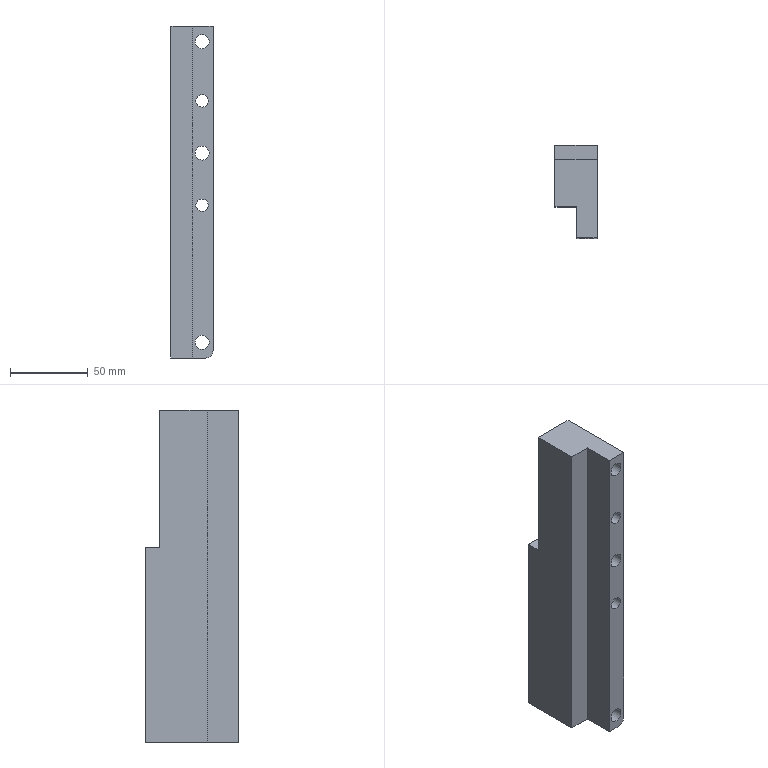Part | STEP file | SLIDE2-PLATE_id562_x_t | 1 solid | 27 faces | box 27 x 59.5 x 213.003 mm | volume 241757 mm3 | plane 18 | cylinder 9 | commonest cylinder face diameters 9 x3 14 x3 8 x2 10 x1
STEP:
#1=CARTESIAN_POINT('',(64.,-40.,62.));
#2=VERTEX_POINT('',#1);
#3=CARTESIAN_POINT('',(64.,-40.,275.003));
#4=VERTEX_POINT('',#3);
#5=CARTESIAN_POINT('',(64.,-40.,275.003));
#6=DIRECTION('',(0.,0.,1.));
#7=VECTOR('',#6,1.);
#8=LINE('',#5,#7);
#9=EDGE_CURVE('',#2,#4,#8,.T.);
#10=ORIENTED_EDGE('',*,*,#9,.T.);
#11=CARTESIAN_POINT('',(50.,-40.,275.003));
#12=VERTEX_POINT('',#11);
#13=CARTESIAN_POINT('',(-89.,-40.,275.003));
#14=DIRECTION('',(1.,0.,0.));
#15=VECTOR('',#14,1.);
#16=LINE('',#13,#15);
#17=EDGE_CURVE('',#12,#4,#16,.T.);
#18=ORIENTED_EDGE('',*,*,#17,.F.);
#19=CARTESIAN_POINT('',(50.,-40.,62.));
#20=VERTEX_POINT('',#19);
#21=CARTESIAN_POINT('',(50.,-40.,47.));
#22=DIRECTION('',(0.,0.,1.));
#23=VECTOR('',#22,1.);
#24=LINE('',#21,#23);
#25=EDGE_CURVE('',#20,#12,#24,.T.);
#26=ORIENTED_EDGE('',*,*,#25,.F.);
#27=CARTESIAN_POINT('',(50.,-40.,62.));
#28=DIRECTION('',(1.,0.,0.));
#29=VECTOR('',#28,1.);
#30=LINE('',#27,#29);
#31=EDGE_CURVE('',#20,#2,#30,.T.);
#32=ORIENTED_EDGE('',*,*,#31,.T.);
#33=EDGE_LOOP('',(#10,#18,#26,#32));
#34=FACE_OUTER_BOUND('',#33,.T.);
#35=CARTESIAN_POINT('',(64.,-40.,275.003));
#36=DIRECTION('',(0.,1.,0.));
#37=DIRECTION('',(0.,0.,1.));
#38=AXIS2_PLACEMENT_3D('',#35,#36,#37);
#39=PLANE('',#38);
#40=ADVANCED_FACE('',(#34),#39,.F.);
#41=ORIENTED_EDGE('',*,*,#9,.F.);
#42=CARTESIAN_POINT('',(64.,-60.,62.));
#43=VERTEX_POINT('',#42);
#44=CARTESIAN_POINT('',(64.,-50.,62.));
#45=DIRECTION('',(0.,-1.,0.));
#46=VECTOR('',#45,1.);
#47=LINE('',#44,#46);
#48=EDGE_CURVE('',#2,#43,#47,.T.);
#49=ORIENTED_EDGE('',*,*,#48,.T.);
#50=CARTESIAN_POINT('',(64.,-60.,275.003));
#51=VERTEX_POINT('',#50);
#52=CARTESIAN_POINT('',(64.,-60.,47.));
#53=DIRECTION('',(0.,0.,-1.));
#54=VECTOR('',#53,1.);
#55=LINE('',#52,#54);
#56=EDGE_CURVE('',#51,#43,#55,.T.);
#57=ORIENTED_EDGE('',*,*,#56,.F.);
#58=CARTESIAN_POINT('',(64.,0.5,275.003));
#59=DIRECTION('',(0.,-1.,0.));
#60=VECTOR('',#59,1.);
#61=LINE('',#58,#60);
#62=EDGE_CURVE('',#4,#51,#61,.T.);
#63=ORIENTED_EDGE('',*,*,#62,.F.);
#64=EDGE_LOOP('',(#41,#49,#57,#63));
#65=FACE_OUTER_BOUND('',#64,.T.);
#66=CARTESIAN_POINT('',(64.,-60.,275.003));
#67=DIRECTION('',(1.,0.,0.));
#68=DIRECTION('',(0.,0.,-1.));
#69=AXIS2_PLACEMENT_3D('',#66,#67,#68);
#70=PLANE('',#69);
#71=ADVANCED_FACE('',(#65),#70,.F.);
#72=CARTESIAN_POINT('',(70.,-60.,76.5));
#73=VERTEX_POINT('',#72);
#74=CARTESIAN_POINT('',(70.,-60.,72.));
#75=DIRECTION('',(0.,1.,0.));
#76=DIRECTION('',(0.,0.,1.));
#77=AXIS2_PLACEMENT_3D('',#74,#75,#76);
#78=CIRCLE('',#77,4.5);
#79=EDGE_CURVE('',#73,#73,#78,.T.);
#80=ORIENTED_EDGE('',*,*,#79,.F.);
#81=EDGE_LOOP('',(#80));
#82=FACE_BOUND('',#81,.T.);
#83=CARTESIAN_POINT('',(70.,-9.5,76.5));
#84=VERTEX_POINT('',#83);
#85=CARTESIAN_POINT('',(70.,-9.5,72.));
#86=DIRECTION('',(0.,-1.,0.));
#87=DIRECTION('',(0.,0.,1.));
#88=AXIS2_PLACEMENT_3D('',#85,#86,#87);
#89=CIRCLE('',#88,4.5);
#90=EDGE_CURVE('',#84,#84,#89,.T.);
#91=ORIENTED_EDGE('',*,*,#90,.F.);
#92=EDGE_LOOP('',(#91));
#93=FACE_BOUND('',#92,.T.);
#94=CARTESIAN_POINT('',(70.,-0.5,72.));
#95=DIRECTION('',(0.,1.,0.));
#96=DIRECTION('',(0.,0.,1.));
#97=AXIS2_PLACEMENT_3D('',#94,#95,#96);
#98=CYLINDRICAL_SURFACE('',#97,4.5);
#99=ADVANCED_FACE('',(#82,#93),#98,.F.);
#100=CARTESIAN_POINT('',(70.,-9.5,65.));
#101=VERTEX_POINT('',#100);
#102=CARTESIAN_POINT('',(70.,-9.5,79.));
#103=VERTEX_POINT('',#102);
#104=CARTESIAN_POINT('',(70.,-9.5,72.));
#105=DIRECTION('',(0.,1.,0.));
#106=DIRECTION('',(0.,0.,1.));
#107=AXIS2_PLACEMENT_3D('',#104,#105,#106);
#108=CIRCLE('',#107,7.);
#109=EDGE_CURVE('',#101,#103,#108,.T.);
#110=ORIENTED_EDGE('',*,*,#109,.F.);
#111=CARTESIAN_POINT('',(70.,-0.5,65.));
#112=VERTEX_POINT('',#111);
#113=CARTESIAN_POINT('',(70.,-0.5,65.));
#114=DIRECTION('',(0.,1.,0.));
#115=VECTOR('',#114,1.);
#116=LINE('',#113,#115);
#117=EDGE_CURVE('',#101,#112,#116,.T.);
#118=ORIENTED_EDGE('',*,*,#117,.T.);
#119=CARTESIAN_POINT('',(70.,-0.5,79.));
#120=VERTEX_POINT('',#119);
#121=CARTESIAN_POINT('',(70.,-0.5,72.));
#122=DIRECTION('',(0.,-1.,0.));
#123=DIRECTION('',(0.,0.,1.));
#124=AXIS2_PLACEMENT_3D('',#121,#122,#123);
#125=CIRCLE('',#124,7.);
#126=EDGE_CURVE('',#120,#112,#125,.T.);
#127=ORIENTED_EDGE('',*,*,#126,.F.);
#128=CARTESIAN_POINT('',(70.,-0.5,79.));
#129=DIRECTION('',(0.,-1.,0.));
#130=VECTOR('',#129,1.);
#131=LINE('',#128,#130);
#132=EDGE_CURVE('',#120,#103,#131,.T.);
#133=ORIENTED_EDGE('',*,*,#132,.T.);
#134=EDGE_LOOP('',(#110,#118,#127,#133));
#135=FACE_OUTER_BOUND('',#134,.T.);
#136=CARTESIAN_POINT('',(70.,-0.5,72.));
#137=DIRECTION('',(0.,1.,0.));
#138=DIRECTION('',(0.,0.,1.));
#139=AXIS2_PLACEMENT_3D('',#136,#137,#138);
#140=CYLINDRICAL_SURFACE('',#139,7.);
#141=ADVANCED_FACE('',(#135),#140,.F.);
#142=CARTESIAN_POINT('',(76.583,-9.5,65.));
#143=VERTEX_POINT('',#142);
#144=CARTESIAN_POINT('',(50.,-9.5,65.));
#145=DIRECTION('',(-1.,0.,0.));
#146=VECTOR('',#145,1.);
#147=LINE('',#144,#146);
#148=EDGE_CURVE('',#143,#101,#147,.T.);
#149=ORIENTED_EDGE('',*,*,#148,.F.);
#150=CARTESIAN_POINT('',(76.583,-0.5,65.));
#151=VERTEX_POINT('',#150);
#152=CARTESIAN_POINT('',(76.583,-0.5,65.));
#153=DIRECTION('',(0.,-1.,0.));
#154=VECTOR('',#153,1.);
#155=LINE('',#152,#154);
#156=EDGE_CURVE('',#151,#143,#155,.T.);
#157=ORIENTED_EDGE('',*,*,#156,.F.);
#158=CARTESIAN_POINT('',(73.,-0.5,65.));
#159=DIRECTION('',(1.,0.,0.));
#160=VECTOR('',#159,1.);
#161=LINE('',#158,#160);
#162=EDGE_CURVE('',#112,#151,#161,.T.);
#163=ORIENTED_EDGE('',*,*,#162,.F.);
#164=ORIENTED_EDGE('',*,*,#117,.F.);
#165=EDGE_LOOP('',(#149,#157,#163,#164));
#166=FACE_OUTER_BOUND('',#165,.T.);
#167=CARTESIAN_POINT('',(77.,-0.5,65.));
#168=DIRECTION('',(0.,0.,-1.));
#169=DIRECTION('',(-1.,0.,0.));
#170=AXIS2_PLACEMENT_3D('',#167,#168,#169);
#171=PLANE('',#170);
#172=ADVANCED_FACE('',(#166),#171,.F.);
#173=CARTESIAN_POINT('',(50.,-0.5,62.));
#174=VERTEX_POINT('',#173);
#175=CARTESIAN_POINT('',(50.,-0.5,62.));
#176=DIRECTION('',(0.,-1.,0.));
#177=VECTOR('',#176,1.);
#178=LINE('',#175,#177);
#179=EDGE_CURVE('',#174,#20,#178,.T.);
#180=ORIENTED_EDGE('',*,*,#179,.F.);
#181=CARTESIAN_POINT('',(72.,-0.5,62.));
#182=VERTEX_POINT('',#181);
#183=CARTESIAN_POINT('',(73.,-0.5,62.));
#184=DIRECTION('',(-1.,0.,0.));
#185=VECTOR('',#184,1.);
#186=LINE('',#183,#185);
#187=EDGE_CURVE('',#182,#174,#186,.T.);
#188=ORIENTED_EDGE('',*,*,#187,.F.);
#189=CARTESIAN_POINT('',(72.,-60.,62.));
#190=VERTEX_POINT('',#189);
#191=CARTESIAN_POINT('',(72.,-0.5,62.));
#192=DIRECTION('',(0.,1.,0.));
#193=VECTOR('',#192,1.);
#194=LINE('',#191,#193);
#195=EDGE_CURVE('',#190,#182,#194,.T.);
#196=ORIENTED_EDGE('',*,*,#195,.F.);
#197=CARTESIAN_POINT('',(58.,-60.,62.));
#198=DIRECTION('',(1.,0.,0.));
#199=VECTOR('',#198,1.);
#200=LINE('',#197,#199);
#201=EDGE_CURVE('',#43,#190,#200,.T.);
#202=ORIENTED_EDGE('',*,*,#201,.F.);
#203=ORIENTED_EDGE('',*,*,#48,.F.);
#204=ORIENTED_EDGE('',*,*,#31,.F.);
#205=EDGE_LOOP('',(#180,#188,#196,#202,#203,#204));
#206=FACE_OUTER_BOUND('',#205,.T.);
#207=CARTESIAN_POINT('',(50.,-50.,62.));
#208=DIRECTION('',(0.,0.,1.));
#209=DIRECTION('',(1.,0.,0.));
#210=AXIS2_PLACEMENT_3D('',#207,#208,#209);
#211=PLANE('',#210);
#212=ADVANCED_FACE('',(#206),#211,.F.);
#213=CARTESIAN_POINT('',(70.,-0.5,164.));
#214=VERTEX_POINT('',#213);
#215=CARTESIAN_POINT('',(70.,-0.5,160.));
#216=DIRECTION('',(0.,-1.,0.));
#217=DIRECTION('',(0.,0.,1.));
#218=AXIS2_PLACEMENT_3D('',#215,#216,#217);
#219=CIRCLE('',#218,4.);
#220=EDGE_CURVE('',#214,#214,#219,.T.);
#221=ORIENTED_EDGE('',*,*,#220,.F.);
#222=EDGE_LOOP('',(#221));
#223=FACE_BOUND('',#222,.T.);
#224=CARTESIAN_POINT('',(70.,-60.,164.));
#225=VERTEX_POINT('',#224);
#226=CARTESIAN_POINT('',(70.,-60.,160.));
#227=DIRECTION('',(0.,1.,0.));
#228=DIRECTION('',(0.,0.,1.));
#229=AXIS2_PLACEMENT_3D('',#226,#227,#228);
#230=CIRCLE('',#229,4.);
#231=EDGE_CURVE('',#225,#225,#230,.T.);
#232=ORIENTED_EDGE('',*,*,#231,.F.);
#233=EDGE_LOOP('',(#232));
#234=FACE_BOUND('',#233,.T.);
#235=CARTESIAN_POINT('',(70.,-0.5,160.));
#236=DIRECTION('',(0.,1.,0.));
#237=DIRECTION('',(0.,0.,1.));
#238=AXIS2_PLACEMENT_3D('',#235,#236,#237);
#239=CYLINDRICAL_SURFACE('',#238,4.);
#240=ADVANCED_FACE('',(#223,#234),#239,.F.);
#241=CARTESIAN_POINT('',(70.,-60.,198.003));
#242=VERTEX_POINT('',#241);
#243=CARTESIAN_POINT('',(70.,-60.,193.503));
#244=DIRECTION('',(0.,1.,0.));
#245=DIRECTION('',(0.,0.,1.));
#246=AXIS2_PLACEMENT_3D('',#243,#244,#245);
#247=CIRCLE('',#246,4.5);
#248=EDGE_CURVE('',#242,#242,#247,.T.);
#249=ORIENTED_EDGE('',*,*,#248,.F.);
#250=EDGE_LOOP('',(#249));
#251=FACE_BOUND('',#250,.T.);
#252=CARTESIAN_POINT('',(70.,-19.5,198.003));
#253=VERTEX_POINT('',#252);
#254=CARTESIAN_POINT('',(70.,-19.5,193.503));
#255=DIRECTION('',(0.,-1.,0.));
#256=DIRECTION('',(0.,0.,1.));
#257=AXIS2_PLACEMENT_3D('',#254,#255,#256);
#258=CIRCLE('',#257,4.5);
#259=EDGE_CURVE('',#253,#253,#258,.T.);
#260=ORIENTED_EDGE('',*,*,#259,.F.);
#261=EDGE_LOOP('',(#260));
#262=FACE_BOUND('',#261,.T.);
#263=CARTESIAN_POINT('',(70.,-0.5,193.503));
#264=DIRECTION('',(0.,1.,0.));
#265=DIRECTION('',(0.,0.,1.));
#266=AXIS2_PLACEMENT_3D('',#263,#264,#265);
#267=CYLINDRICAL_SURFACE('',#266,4.5);
#268=ADVANCED_FACE('',(#251,#262),#267,.F.);
#269=CARTESIAN_POINT('',(70.,-60.,269.503));
#270=VERTEX_POINT('',#269);
#271=CARTESIAN_POINT('',(70.,-60.,265.003));
#272=DIRECTION('',(0.,1.,0.));
#273=DIRECTION('',(0.,0.,1.));
#274=AXIS2_PLACEMENT_3D('',#271,#272,#273);
#275=CIRCLE('',#274,4.5);
#276=EDGE_CURVE('',#270,#270,#275,.T.);
#277=ORIENTED_EDGE('',*,*,#276,.F.);
#278=EDGE_LOOP('',(#277));
#279=FACE_BOUND('',#278,.T.);
#280=CARTESIAN_POINT('',(70.,-19.5,269.503));
#281=VERTEX_POINT('',#280);
#282=CARTESIAN_POINT('',(70.,-19.5,265.003));
#283=DIRECTION('',(0.,-1.,0.));
#284=DIRECTION('',(0.,0.,1.));
#285=AXIS2_PLACEMENT_3D('',#282,#283,#284);
#286=CIRCLE('',#285,4.5);
#287=EDGE_CURVE('',#281,#281,#286,.T.);
#288=ORIENTED_EDGE('',*,*,#287,.F.);
#289=EDGE_LOOP('',(#288));
#290=FACE_BOUND('',#289,.T.);
#291=CARTESIAN_POINT('',(70.,-0.5,265.003));
#292=DIRECTION('',(0.,1.,0.));
#293=DIRECTION('',(0.,0.,1.));
#294=AXIS2_PLACEMENT_3D('',#291,#292,#293);
#295=CYLINDRICAL_SURFACE('',#294,4.5);
#296=ADVANCED_FACE('',(#279,#290),#295,.F.);
#297=CARTESIAN_POINT('',(70.,-19.5,258.003));
#298=VERTEX_POINT('',#297);
#299=CARTESIAN_POINT('',(70.,-19.5,272.003));
#300=VERTEX_POINT('',#299);
#301=CARTESIAN_POINT('',(70.,-19.5,265.003));
#302=DIRECTION('',(0.,1.,0.));
#303=DIRECTION('',(0.,0.,1.));
#304=AXIS2_PLACEMENT_3D('',#301,#302,#303);
#305=CIRCLE('',#304,7.);
#306=EDGE_CURVE('',#298,#300,#305,.T.);
#307=ORIENTED_EDGE('',*,*,#306,.F.);
#308=CARTESIAN_POINT('',(70.,-9.5,258.003));
#309=VERTEX_POINT('',#308);
#310=CARTESIAN_POINT('',(70.,-0.5,258.003));
#311=DIRECTION('',(0.,1.,0.));
#312=VECTOR('',#311,1.);
#313=LINE('',#310,#312);
#314=EDGE_CURVE('',#298,#309,#313,.T.);
#315=ORIENTED_EDGE('',*,*,#314,.T.);
#316=CARTESIAN_POINT('',(70.,-9.5,272.003));
#317=VERTEX_POINT('',#316);
#318=CARTESIAN_POINT('',(70.,-9.5,265.003));
#319=DIRECTION('',(0.,-1.,0.));
#320=DIRECTION('',(0.,0.,1.));
#321=AXIS2_PLACEMENT_3D('',#318,#319,#320);
#322=CIRCLE('',#321,7.);
#323=EDGE_CURVE('',#317,#309,#322,.T.);
#324=ORIENTED_EDGE('',*,*,#323,.F.);
#325=CARTESIAN_POINT('',(70.,-0.5,272.003));
#326=DIRECTION('',(0.,-1.,0.));
#327=VECTOR('',#326,1.);
#328=LINE('',#325,#327);
#329=EDGE_CURVE('',#317,#300,#328,.T.);
#330=ORIENTED_EDGE('',*,*,#329,.T.);
#331=EDGE_LOOP('',(#307,#315,#324,#330));
#332=FACE_OUTER_BOUND('',#331,.T.);
#333=CARTESIAN_POINT('',(70.,-0.5,265.003));
#334=DIRECTION('',(0.,1.,0.));
#335=DIRECTION('',(0.,0.,1.));
#336=AXIS2_PLACEMENT_3D('',#333,#334,#335);
#337=CYLINDRICAL_SURFACE('',#336,7.);
#338=ADVANCED_FACE('',(#332),#337,.F.);
#339=CARTESIAN_POINT('',(70.,-19.5,186.503));
#340=VERTEX_POINT('',#339);
#341=CARTESIAN_POINT('',(70.,-19.5,200.503));
#342=VERTEX_POINT('',#341);
#343=CARTESIAN_POINT('',(70.,-19.5,193.503));
#344=DIRECTION('',(0.,1.,0.));
#345=DIRECTION('',(0.,0.,1.));
#346=AXIS2_PLACEMENT_3D('',#343,#344,#345);
#347=CIRCLE('',#346,7.);
#348=EDGE_CURVE('',#340,#342,#347,.T.);
#349=ORIENTED_EDGE('',*,*,#348,.F.);
#350=CARTESIAN_POINT('',(70.,-9.5,186.503));
#351=VERTEX_POINT('',#350);
#352=CARTESIAN_POINT('',(70.,-0.5,186.503));
#353=DIRECTION('',(0.,1.,0.));
#354=VECTOR('',#353,1.);
#355=LINE('',#352,#354);
#356=EDGE_CURVE('',#340,#351,#355,.T.);
#357=ORIENTED_EDGE('',*,*,#356,.T.);
#358=CARTESIAN_POINT('',(70.,-9.5,200.503));
#359=VERTEX_POINT('',#358);
#360=CARTESIAN_POINT('',(70.,-9.5,193.503));
#361=DIRECTION('',(0.,-1.,0.));
#362=DIRECTION('',(0.,0.,1.));
#363=AXIS2_PLACEMENT_3D('',#360,#361,#362);
#364=CIRCLE('',#363,7.);
#365=EDGE_CURVE('',#359,#351,#364,.T.);
#366=ORIENTED_EDGE('',*,*,#365,.F.);
#367=CARTESIAN_POINT('',(70.,-0.5,200.503));
#368=DIRECTION('',(0.,-1.,0.));
#369=VECTOR('',#368,1.);
#370=LINE('',#367,#369);
#371=EDGE_CURVE('',#359,#342,#370,.T.);
#372=ORIENTED_EDGE('',*,*,#371,.T.);
#373=EDGE_LOOP('',(#349,#357,#366,#372));
#374=FACE_OUTER_BOUND('',#373,.T.);
#375=CARTESIAN_POINT('',(70.,-0.5,193.503));
#376=DIRECTION('',(0.,1.,0.));
#377=DIRECTION('',(0.,0.,1.));
#378=AXIS2_PLACEMENT_3D('',#375,#376,#377);
#379=CYLINDRICAL_SURFACE('',#378,7.);
#380=ADVANCED_FACE('',(#374),#379,.F.);
#381=CARTESIAN_POINT('',(50.,-9.5,275.003));
#382=VERTEX_POINT('',#381);
#383=CARTESIAN_POINT('',(50.,0.5,275.003));
#384=DIRECTION('',(0.,-1.,0.));
#385=VECTOR('',#384,1.);
#386=LINE('',#383,#385);
#387=EDGE_CURVE('',#382,#12,#386,.T.);
#388=ORIENTED_EDGE('',*,*,#387,.F.);
#389=CARTESIAN_POINT('',(50.,-9.5,186.503));
#390=VERTEX_POINT('',#389);
#391=CARTESIAN_POINT('',(50.,-9.5,47.));
#392=DIRECTION('',(0.,0.,1.));
#393=VECTOR('',#392,1.);
#394=LINE('',#391,#393);
#395=EDGE_CURVE('',#390,#382,#394,.T.);
#396=ORIENTED_EDGE('',*,*,#395,.F.);
#397=CARTESIAN_POINT('',(50.,-0.5,186.503));
#398=VERTEX_POINT('',#397);
#399=CARTESIAN_POINT('',(50.,-0.5,186.503));
#400=DIRECTION('',(0.,1.,0.));
#401=VECTOR('',#400,1.);
#402=LINE('',#399,#401);
#403=EDGE_CURVE('',#390,#398,#402,.T.);
#404=ORIENTED_EDGE('',*,*,#403,.T.);
#405=CARTESIAN_POINT('',(50.,-0.5,47.));
#406=DIRECTION('',(0.,0.,1.));
#407=VECTOR('',#406,1.);
#408=LINE('',#405,#407);
#409=EDGE_CURVE('',#174,#398,#408,.T.);
#410=ORIENTED_EDGE('',*,*,#409,.F.);
#411=ORIENTED_EDGE('',*,*,#179,.T.);
#412=ORIENTED_EDGE('',*,*,#25,.T.);
#413=EDGE_LOOP('',(#388,#396,#404,#410,#411,#412));
#414=FACE_OUTER_BOUND('',#413,.T.);
#415=CARTESIAN_POINT('',(50.,-0.5,47.));
#416=DIRECTION('',(-1.,0.,0.));
#417=DIRECTION('',(0.,0.,1.));
#418=AXIS2_PLACEMENT_3D('',#415,#416,#417);
#419=PLANE('',#418);
#420=ADVANCED_FACE('',(#414),#419,.T.);
#421=CARTESIAN_POINT('',(70.,-60.,231.003));
#422=VERTEX_POINT('',#421);
#423=CARTESIAN_POINT('',(70.,-60.,227.003));
#424=DIRECTION('',(0.,1.,0.));
#425=DIRECTION('',(0.,0.,1.));
#426=AXIS2_PLACEMENT_3D('',#423,#424,#425);
#427=CIRCLE('',#426,4.);
#428=EDGE_CURVE('',#422,#422,#427,.T.);
#429=ORIENTED_EDGE('',*,*,#428,.F.);
#430=EDGE_LOOP('',(#429));
#431=FACE_BOUND('',#430,.T.);
#432=CARTESIAN_POINT('',(70.,-9.5,231.003));
#433=VERTEX_POINT('',#432);
#434=CARTESIAN_POINT('',(70.,-9.5,227.003));
#435=DIRECTION('',(0.,-1.,0.));
#436=DIRECTION('',(0.,0.,1.));
#437=AXIS2_PLACEMENT_3D('',#434,#435,#436);
#438=CIRCLE('',#437,4.);
#439=EDGE_CURVE('',#433,#433,#438,.T.);
#440=ORIENTED_EDGE('',*,*,#439,.F.);
#441=EDGE_LOOP('',(#440));
#442=FACE_BOUND('',#441,.T.);
#443=CARTESIAN_POINT('',(70.,-0.5,227.003));
#444=DIRECTION('',(0.,1.,0.));
#445=DIRECTION('',(0.,0.,1.));
#446=AXIS2_PLACEMENT_3D('',#443,#444,#445);
#447=CYLINDRICAL_SURFACE('',#446,4.);
#448=ADVANCED_FACE('',(#431,#442),#447,.F.);
#449=CARTESIAN_POINT('',(77.,-9.5,275.003));
#450=VERTEX_POINT('',#449);
#451=CARTESIAN_POINT('',(77.,-60.,275.003));
#452=VERTEX_POINT('',#451);
#453=CARTESIAN_POINT('',(77.,-0.5,275.003));
#454=DIRECTION('',(0.,-1.,0.));
#455=VECTOR('',#454,1.);
#456=LINE('',#453,#455);
#457=EDGE_CURVE('',#450,#452,#456,.T.);
#458=ORIENTED_EDGE('',*,*,#457,.F.);
#459=CARTESIAN_POINT('',(50.,-9.5,275.003));
#460=DIRECTION('',(1.,0.,0.));
#461=VECTOR('',#460,1.);
#462=LINE('',#459,#461);
#463=EDGE_CURVE('',#382,#450,#462,.T.);
#464=ORIENTED_EDGE('',*,*,#463,.F.);
#465=ORIENTED_EDGE('',*,*,#387,.T.);
#466=ORIENTED_EDGE('',*,*,#17,.T.);
#467=ORIENTED_EDGE('',*,*,#62,.T.);
#468=CARTESIAN_POINT('',(58.,-60.,275.003));
#469=DIRECTION('',(-1.,0.,0.));
#470=VECTOR('',#469,1.);
#471=LINE('',#468,#470);
#472=EDGE_CURVE('',#452,#51,#471,.T.);
#473=ORIENTED_EDGE('',*,*,#472,.F.);
#474=EDGE_LOOP('',(#458,#464,#465,#466,#467,#473));
#475=FACE_OUTER_BOUND('',#474,.T.);
#476=CARTESIAN_POINT('',(-89.,0.5,275.003));
#477=DIRECTION('',(0.,0.,1.));
#478=DIRECTION('',(1.,0.,0.));
#479=AXIS2_PLACEMENT_3D('',#476,#477,#478);
#480=PLANE('',#479);
#481=ADVANCED_FACE('',(#475),#480,.T.);
#482=ORIENTED_EDGE('',*,*,#248,.T.);
#483=EDGE_LOOP('',(#482));
#484=FACE_BOUND('',#483,.T.);
#485=ORIENTED_EDGE('',*,*,#276,.T.);
#486=EDGE_LOOP('',(#485));
#487=FACE_BOUND('',#486,.T.);
#488=ORIENTED_EDGE('',*,*,#428,.T.);
#489=EDGE_LOOP('',(#488));
#490=FACE_BOUND('',#489,.T.);
#491=ORIENTED_EDGE('',*,*,#231,.T.);
#492=EDGE_LOOP('',(#491));
#493=FACE_BOUND('',#492,.T.);
#494=ORIENTED_EDGE('',*,*,#79,.T.);
#495=EDGE_LOOP('',(#494));
#496=FACE_BOUND('',#495,.T.);
#497=ORIENTED_EDGE('',*,*,#472,.T.);
#498=ORIENTED_EDGE('',*,*,#56,.T.);
#499=ORIENTED_EDGE('',*,*,#201,.T.);
#500=CARTESIAN_POINT('',(77.,-60.,67.));
#501=VERTEX_POINT('',#500);
#502=CARTESIAN_POINT('',(72.,-60.,67.));
#503=DIRECTION('',(0.,1.,0.));
#504=DIRECTION('',(0.,0.,-1.));
#505=AXIS2_PLACEMENT_3D('',#502,#503,#504);
#506=CIRCLE('',#505,5.);
#507=EDGE_CURVE('',#501,#190,#506,.T.);
#508=ORIENTED_EDGE('',*,*,#507,.F.);
#509=CARTESIAN_POINT('',(77.,-60.,67.));
#510=DIRECTION('',(0.,0.,-1.));
#511=VECTOR('',#510,1.);
#512=LINE('',#509,#511);
#513=EDGE_CURVE('',#452,#501,#512,.T.);
#514=ORIENTED_EDGE('',*,*,#513,.F.);
#515=EDGE_LOOP('',(#497,#498,#499,#508,#514));
#516=FACE_BOUND('',#515,.T.);
#517=CARTESIAN_POINT('',(58.,-60.,47.));
#518=DIRECTION('',(0.,-1.,0.));
#519=DIRECTION('',(0.,0.,-1.));
#520=AXIS2_PLACEMENT_3D('',#517,#518,#519);
#521=PLANE('',#520);
#522=ADVANCED_FACE('',(#484,#487,#490,#493,#496,#516),#521,.T.);
#523=ORIENTED_EDGE('',*,*,#156,.T.);
#524=CARTESIAN_POINT('',(77.,-9.5,67.));
#525=VERTEX_POINT('',#524);
#526=CARTESIAN_POINT('',(72.,-9.5,67.));
#527=DIRECTION('',(0.,1.,0.));
#528=DIRECTION('',(0.,0.,-1.));
#529=AXIS2_PLACEMENT_3D('',#526,#527,#528);
#530=CIRCLE('',#529,5.);
#531=EDGE_CURVE('',#525,#143,#530,.T.);
#532=ORIENTED_EDGE('',*,*,#531,.F.);
#533=CARTESIAN_POINT('',(77.,-0.5,67.));
#534=DIRECTION('',(0.,1.,0.));
#535=VECTOR('',#534,1.);
#536=LINE('',#533,#535);
#537=EDGE_CURVE('',#501,#525,#536,.T.);
#538=ORIENTED_EDGE('',*,*,#537,.F.);
#539=ORIENTED_EDGE('',*,*,#507,.T.);
#540=ORIENTED_EDGE('',*,*,#195,.T.);
#541=CARTESIAN_POINT('',(72.,-0.5,67.));
#542=DIRECTION('',(0.,1.,0.));
#543=DIRECTION('',(0.,0.,-1.));
#544=AXIS2_PLACEMENT_3D('',#541,#542,#543);
#545=CIRCLE('',#544,5.);
#546=EDGE_CURVE('',#151,#182,#545,.T.);
#547=ORIENTED_EDGE('',*,*,#546,.F.);
#548=EDGE_LOOP('',(#523,#532,#538,#539,#540,#547));
#549=FACE_OUTER_BOUND('',#548,.T.);
#550=CARTESIAN_POINT('',(72.,-0.5,67.));
#551=DIRECTION('',(0.,-1.,0.));
#552=DIRECTION('',(0.,0.,-1.));
#553=AXIS2_PLACEMENT_3D('',#550,#551,#552);
#554=CYLINDRICAL_SURFACE('',#553,5.);
#555=ADVANCED_FACE('',(#549),#554,.T.);
#556=ORIENTED_EDGE('',*,*,#90,.T.);
#557=EDGE_LOOP('',(#556));
#558=FACE_BOUND('',#557,.T.);
#559=CARTESIAN_POINT('',(77.,-9.5,79.));
#560=VERTEX_POINT('',#559);
#561=CARTESIAN_POINT('',(77.,-9.5,67.));
#562=DIRECTION('',(0.,0.,1.));
#563=VECTOR('',#562,1.);
#564=LINE('',#561,#563);
#565=EDGE_CURVE('',#525,#560,#564,.T.);
#566=ORIENTED_EDGE('',*,*,#565,.F.);
#567=ORIENTED_EDGE('',*,*,#531,.T.);
#568=ORIENTED_EDGE('',*,*,#148,.T.);
#569=ORIENTED_EDGE('',*,*,#109,.T.);
#570=CARTESIAN_POINT('',(70.,-9.5,79.));
#571=DIRECTION('',(1.,0.,0.));
#572=VECTOR('',#571,1.);
#573=LINE('',#570,#572);
#574=EDGE_CURVE('',#103,#560,#573,.T.);
#575=ORIENTED_EDGE('',*,*,#574,.T.);
#576=EDGE_LOOP('',(#566,#567,#568,#569,#575));
#577=FACE_BOUND('',#576,.T.);
#578=CARTESIAN_POINT('',(50.,-9.5,47.));
#579=DIRECTION('',(0.,1.,0.));
#580=DIRECTION('',(0.,0.,1.));
#581=AXIS2_PLACEMENT_3D('',#578,#579,#580);
#582=PLANE('',#581);
#583=ADVANCED_FACE('',(#558,#577),#582,.T.);
#584=ORIENTED_EDGE('',*,*,#574,.F.);
#585=ORIENTED_EDGE('',*,*,#132,.F.);
#586=CARTESIAN_POINT('',(77.,-0.5,79.));
#587=VERTEX_POINT('',#586);
#588=CARTESIAN_POINT('',(73.,-0.5,79.));
#589=DIRECTION('',(-1.,0.,0.));
#590=VECTOR('',#589,1.);
#591=LINE('',#588,#590);
#592=EDGE_CURVE('',#587,#120,#591,.T.);
#593=ORIENTED_EDGE('',*,*,#592,.F.);
#594=CARTESIAN_POINT('',(77.,-0.5,79.));
#595=DIRECTION('',(0.,1.,0.));
#596=VECTOR('',#595,1.);
#597=LINE('',#594,#596);
#598=EDGE_CURVE('',#560,#587,#597,.T.);
#599=ORIENTED_EDGE('',*,*,#598,.F.);
#600=EDGE_LOOP('',(#584,#585,#593,#599));
#601=FACE_OUTER_BOUND('',#600,.T.);
#602=CARTESIAN_POINT('',(70.,-0.5,79.));
#603=DIRECTION('',(0.,0.,1.));
#604=DIRECTION('',(1.,0.,0.));
#605=AXIS2_PLACEMENT_3D('',#602,#603,#604);
#606=PLANE('',#605);
#607=ADVANCED_FACE('',(#601),#606,.F.);
#608=ORIENTED_EDGE('',*,*,#220,.T.);
#609=EDGE_LOOP('',(#608));
#610=FACE_BOUND('',#609,.T.);
#611=ORIENTED_EDGE('',*,*,#409,.T.);
#612=CARTESIAN_POINT('',(77.,-0.5,186.503));
#613=VERTEX_POINT('',#612);
#614=CARTESIAN_POINT('',(77.,-0.5,186.503));
#615=DIRECTION('',(1.,0.,0.));
#616=VECTOR('',#615,1.);
#617=LINE('',#614,#616);
#618=EDGE_CURVE('',#398,#613,#617,.T.);
#619=ORIENTED_EDGE('',*,*,#618,.T.);
#620=CARTESIAN_POINT('',(77.,-0.5,67.));
#621=DIRECTION('',(0.,0.,1.));
#622=VECTOR('',#621,1.);
#623=LINE('',#620,#622);
#624=EDGE_CURVE('',#587,#613,#623,.T.);
#625=ORIENTED_EDGE('',*,*,#624,.F.);
#626=ORIENTED_EDGE('',*,*,#592,.T.);
#627=ORIENTED_EDGE('',*,*,#126,.T.);
#628=ORIENTED_EDGE('',*,*,#162,.T.);
#629=ORIENTED_EDGE('',*,*,#546,.T.);
#630=ORIENTED_EDGE('',*,*,#187,.T.);
#631=EDGE_LOOP('',(#611,#619,#625,#626,#627,#628,#629,#630));
#632=FACE_BOUND('',#631,.T.);
#633=CARTESIAN_POINT('',(73.,-0.5,47.));
#634=DIRECTION('',(0.,1.,0.));
#635=DIRECTION('',(0.,0.,1.));
#636=AXIS2_PLACEMENT_3D('',#633,#634,#635);
#637=PLANE('',#636);
#638=ADVANCED_FACE('',(#610,#632),#637,.T.);
#639=CARTESIAN_POINT('',(77.,-19.5,186.503));
#640=VERTEX_POINT('',#639);
#641=CARTESIAN_POINT('',(77.,-0.5,186.503));
#642=DIRECTION('',(0.,-1.,0.));
#643=VECTOR('',#642,1.);
#644=LINE('',#641,#643);
#645=EDGE_CURVE('',#613,#640,#644,.T.);
#646=ORIENTED_EDGE('',*,*,#645,.F.);
#647=ORIENTED_EDGE('',*,*,#618,.F.);
#648=ORIENTED_EDGE('',*,*,#403,.F.);
#649=CARTESIAN_POINT('',(50.,-9.5,186.503));
#650=DIRECTION('',(-1.,0.,0.));
#651=VECTOR('',#650,1.);
#652=LINE('',#649,#651);
#653=EDGE_CURVE('',#351,#390,#652,.T.);
#654=ORIENTED_EDGE('',*,*,#653,.F.);
#655=ORIENTED_EDGE('',*,*,#356,.F.);
#656=CARTESIAN_POINT('',(50.,-19.5,186.503));
#657=DIRECTION('',(-1.,0.,0.));
#658=VECTOR('',#657,1.);
#659=LINE('',#656,#658);
#660=EDGE_CURVE('',#640,#340,#659,.T.);
#661=ORIENTED_EDGE('',*,*,#660,.F.);
#662=EDGE_LOOP('',(#646,#647,#648,#654,#655,#661));
#663=FACE_OUTER_BOUND('',#662,.T.);
#664=CARTESIAN_POINT('',(77.,-0.5,186.503));
#665=DIRECTION('',(0.,0.,-1.));
#666=DIRECTION('',(-1.,0.,0.));
#667=AXIS2_PLACEMENT_3D('',#664,#665,#666);
#668=PLANE('',#667);
#669=ADVANCED_FACE('',(#663),#668,.F.);
#670=ORIENTED_EDGE('',*,*,#259,.T.);
#671=EDGE_LOOP('',(#670));
#672=FACE_BOUND('',#671,.T.);
#673=CARTESIAN_POINT('',(77.,-19.5,200.503));
#674=VERTEX_POINT('',#673);
#675=CARTESIAN_POINT('',(70.,-19.5,200.503));
#676=DIRECTION('',(1.,0.,0.));
#677=VECTOR('',#676,1.);
#678=LINE('',#675,#677);
#679=EDGE_CURVE('',#342,#674,#678,.T.);
#680=ORIENTED_EDGE('',*,*,#679,.T.);
#681=CARTESIAN_POINT('',(77.,-19.5,67.));
#682=DIRECTION('',(0.,0.,1.));
#683=VECTOR('',#682,1.);
#684=LINE('',#681,#683);
#685=EDGE_CURVE('',#640,#674,#684,.T.);
#686=ORIENTED_EDGE('',*,*,#685,.F.);
#687=ORIENTED_EDGE('',*,*,#660,.T.);
#688=ORIENTED_EDGE('',*,*,#348,.T.);
#689=EDGE_LOOP('',(#680,#686,#687,#688));
#690=FACE_BOUND('',#689,.T.);
#691=CARTESIAN_POINT('',(50.,-19.5,47.));
#692=DIRECTION('',(0.,1.,0.));
#693=DIRECTION('',(0.,0.,1.));
#694=AXIS2_PLACEMENT_3D('',#691,#692,#693);
#695=PLANE('',#694);
#696=ADVANCED_FACE('',(#672,#690),#695,.T.);
#697=ORIENTED_EDGE('',*,*,#679,.F.);
#698=ORIENTED_EDGE('',*,*,#371,.F.);
#699=CARTESIAN_POINT('',(77.,-9.5,200.503));
#700=VERTEX_POINT('',#699);
#701=CARTESIAN_POINT('',(50.,-9.5,200.503));
#702=DIRECTION('',(-1.,0.,0.));
#703=VECTOR('',#702,1.);
#704=LINE('',#701,#703);
#705=EDGE_CURVE('',#700,#359,#704,.T.);
#706=ORIENTED_EDGE('',*,*,#705,.F.);
#707=CARTESIAN_POINT('',(77.,-0.5,200.503));
#708=DIRECTION('',(0.,1.,0.));
#709=VECTOR('',#708,1.);
#710=LINE('',#707,#709);
#711=EDGE_CURVE('',#674,#700,#710,.T.);
#712=ORIENTED_EDGE('',*,*,#711,.F.);
#713=EDGE_LOOP('',(#697,#698,#706,#712));
#714=FACE_OUTER_BOUND('',#713,.T.);
#715=CARTESIAN_POINT('',(70.,-0.5,200.503));
#716=DIRECTION('',(0.,0.,1.));
#717=DIRECTION('',(1.,0.,0.));
#718=AXIS2_PLACEMENT_3D('',#715,#716,#717);
#719=PLANE('',#718);
#720=ADVANCED_FACE('',(#714),#719,.F.);
#721=CARTESIAN_POINT('',(77.,-19.5,258.003));
#722=VERTEX_POINT('',#721);
#723=CARTESIAN_POINT('',(50.,-19.5,258.003));
#724=DIRECTION('',(-1.,0.,0.));
#725=VECTOR('',#724,1.);
#726=LINE('',#723,#725);
#727=EDGE_CURVE('',#722,#298,#726,.T.);
#728=ORIENTED_EDGE('',*,*,#727,.F.);
#729=CARTESIAN_POINT('',(77.,-9.5,258.003));
#730=VERTEX_POINT('',#729);
#731=CARTESIAN_POINT('',(77.,-0.5,258.003));
#732=DIRECTION('',(0.,-1.,0.));
#733=VECTOR('',#732,1.);
#734=LINE('',#731,#733);
#735=EDGE_CURVE('',#730,#722,#734,.T.);
#736=ORIENTED_EDGE('',*,*,#735,.F.);
#737=CARTESIAN_POINT('',(50.,-9.5,258.003));
#738=DIRECTION('',(1.,0.,0.));
#739=VECTOR('',#738,1.);
#740=LINE('',#737,#739);
#741=EDGE_CURVE('',#309,#730,#740,.T.);
#742=ORIENTED_EDGE('',*,*,#741,.F.);
#743=ORIENTED_EDGE('',*,*,#314,.F.);
#744=EDGE_LOOP('',(#728,#736,#742,#743));
#745=FACE_OUTER_BOUND('',#744,.T.);
#746=CARTESIAN_POINT('',(77.,-0.5,258.003));
#747=DIRECTION('',(0.,0.,-1.));
#748=DIRECTION('',(-1.,0.,0.));
#749=AXIS2_PLACEMENT_3D('',#746,#747,#748);
#750=PLANE('',#749);
#751=ADVANCED_FACE('',(#745),#750,.F.);
#752=ORIENTED_EDGE('',*,*,#287,.T.);
#753=EDGE_LOOP('',(#752));
#754=FACE_BOUND('',#753,.T.);
#755=CARTESIAN_POINT('',(77.,-19.5,272.003));
#756=VERTEX_POINT('',#755);
#757=CARTESIAN_POINT('',(70.,-19.5,272.003));
#758=DIRECTION('',(1.,0.,0.));
#759=VECTOR('',#758,1.);
#760=LINE('',#757,#759);
#761=EDGE_CURVE('',#300,#756,#760,.T.);
#762=ORIENTED_EDGE('',*,*,#761,.T.);
#763=CARTESIAN_POINT('',(77.,-19.5,67.));
#764=DIRECTION('',(0.,0.,1.));
#765=VECTOR('',#764,1.);
#766=LINE('',#763,#765);
#767=EDGE_CURVE('',#722,#756,#766,.T.);
#768=ORIENTED_EDGE('',*,*,#767,.F.);
#769=ORIENTED_EDGE('',*,*,#727,.T.);
#770=ORIENTED_EDGE('',*,*,#306,.T.);
#771=EDGE_LOOP('',(#762,#768,#769,#770));
#772=FACE_BOUND('',#771,.T.);
#773=CARTESIAN_POINT('',(50.,-19.5,47.));
#774=DIRECTION('',(0.,1.,0.));
#775=DIRECTION('',(0.,0.,1.));
#776=AXIS2_PLACEMENT_3D('',#773,#774,#775);
#777=PLANE('',#776);
#778=ADVANCED_FACE('',(#754,#772),#777,.T.);
#779=ORIENTED_EDGE('',*,*,#761,.F.);
#780=ORIENTED_EDGE('',*,*,#329,.F.);
#781=CARTESIAN_POINT('',(77.,-9.5,272.003));
#782=VERTEX_POINT('',#781);
#783=CARTESIAN_POINT('',(50.,-9.5,272.003));
#784=DIRECTION('',(-1.,0.,0.));
#785=VECTOR('',#784,1.);
#786=LINE('',#783,#785);
#787=EDGE_CURVE('',#782,#317,#786,.T.);
#788=ORIENTED_EDGE('',*,*,#787,.F.);
#789=CARTESIAN_POINT('',(77.,-0.5,272.003));
#790=DIRECTION('',(0.,1.,0.));
#791=VECTOR('',#790,1.);
#792=LINE('',#789,#791);
#793=EDGE_CURVE('',#756,#782,#792,.T.);
#794=ORIENTED_EDGE('',*,*,#793,.F.);
#795=EDGE_LOOP('',(#779,#780,#788,#794));
#796=FACE_OUTER_BOUND('',#795,.T.);
#797=CARTESIAN_POINT('',(70.,-0.5,272.003));
#798=DIRECTION('',(0.,0.,1.));
#799=DIRECTION('',(1.,0.,0.));
#800=AXIS2_PLACEMENT_3D('',#797,#798,#799);
#801=PLANE('',#800);
#802=ADVANCED_FACE('',(#796),#801,.F.);
#803=ORIENTED_EDGE('',*,*,#439,.T.);
#804=EDGE_LOOP('',(#803));
#805=FACE_BOUND('',#804,.T.);
#806=ORIENTED_EDGE('',*,*,#653,.T.);
#807=ORIENTED_EDGE('',*,*,#395,.T.);
#808=ORIENTED_EDGE('',*,*,#463,.T.);
#809=CARTESIAN_POINT('',(77.,-9.5,67.));
#810=DIRECTION('',(0.,0.,1.));
#811=VECTOR('',#810,1.);
#812=LINE('',#809,#811);
#813=EDGE_CURVE('',#782,#450,#812,.T.);
#814=ORIENTED_EDGE('',*,*,#813,.F.);
#815=ORIENTED_EDGE('',*,*,#787,.T.);
#816=ORIENTED_EDGE('',*,*,#323,.T.);
#817=ORIENTED_EDGE('',*,*,#741,.T.);
#818=CARTESIAN_POINT('',(77.,-9.5,67.));
#819=DIRECTION('',(0.,0.,1.));
#820=VECTOR('',#819,1.);
#821=LINE('',#818,#820);
#822=EDGE_CURVE('',#700,#730,#821,.T.);
#823=ORIENTED_EDGE('',*,*,#822,.F.);
#824=ORIENTED_EDGE('',*,*,#705,.T.);
#825=ORIENTED_EDGE('',*,*,#365,.T.);
#826=EDGE_LOOP('',(#806,#807,#808,#814,#815,#816,#817,#823,#824,#825));
#827=FACE_BOUND('',#826,.T.);
#828=CARTESIAN_POINT('',(50.,-9.5,47.));
#829=DIRECTION('',(0.,1.,0.));
#830=DIRECTION('',(0.,0.,1.));
#831=AXIS2_PLACEMENT_3D('',#828,#829,#830);
#832=PLANE('',#831);
#833=ADVANCED_FACE('',(#805,#827),#832,.T.);
#834=ORIENTED_EDGE('',*,*,#793,.T.);
#835=ORIENTED_EDGE('',*,*,#813,.T.);
#836=ORIENTED_EDGE('',*,*,#457,.T.);
#837=ORIENTED_EDGE('',*,*,#513,.T.);
#838=ORIENTED_EDGE('',*,*,#537,.T.);
#839=ORIENTED_EDGE('',*,*,#565,.T.);
#840=ORIENTED_EDGE('',*,*,#598,.T.);
#841=ORIENTED_EDGE('',*,*,#624,.T.);
#842=ORIENTED_EDGE('',*,*,#645,.T.);
#843=ORIENTED_EDGE('',*,*,#685,.T.);
#844=ORIENTED_EDGE('',*,*,#711,.T.);
#845=ORIENTED_EDGE('',*,*,#822,.T.);
#846=ORIENTED_EDGE('',*,*,#735,.T.);
#847=ORIENTED_EDGE('',*,*,#767,.T.);
#848=EDGE_LOOP('',(#834,#835,#836,#837,#838,#839,#840,#841,#842,#843,#844,#845,#846,#847));
#849=FACE_OUTER_BOUND('',#848,.T.);
#850=CARTESIAN_POINT('',(77.,-0.5,67.));
#851=DIRECTION('',(1.,0.,0.));
#852=DIRECTION('',(0.,0.,-1.));
#853=AXIS2_PLACEMENT_3D('',#850,#851,#852);
#854=PLANE('',#853);
#855=ADVANCED_FACE('',(#849),#854,.T.);
#856=CLOSED_SHELL('',(#40,#71,#99,#141,#172,#212,#240,#268,#296,#338,#380,#420,#448,#481,#522,#555,#583,#607,#638,#669,#696,#720,#751,#778,#802,#833,#855));
#857=MANIFOLD_SOLID_BREP('',#856);
#858=(LENGTH_UNIT()NAMED_UNIT(*)SI_UNIT(.MILLI.,.METRE.));
#859=UNCERTAINTY_MEASURE_WITH_UNIT(LENGTH_MEASURE(0.00004123),#858,'','');
#860=(NAMED_UNIT(*)PLANE_ANGLE_UNIT()SI_UNIT($,.RADIAN.));
#861=PLANE_ANGLE_MEASURE_WITH_UNIT(PLANE_ANGLE_MEASURE(0.01745),#860);
#862=DIMENSIONAL_EXPONENTS(0.,0.,0.,0.,0.,0.,0.);
#863=(CONVERSION_BASED_UNIT('DEGREE',#861)NAMED_UNIT(#862)PLANE_ANGLE_UNIT());
#864=(NAMED_UNIT(*)SI_UNIT($,.STERADIAN.)SOLID_ANGLE_UNIT());
#865=(GEOMETRIC_REPRESENTATION_CONTEXT(3)GLOBAL_UNCERTAINTY_ASSIGNED_CONTEXT((#859))GLOBAL_UNIT_ASSIGNED_CONTEXT((#858,#863,#864))REPRESENTATION_CONTEXT('',''));
#866=ADVANCED_BREP_SHAPE_REPRESENTATION('',(#857),#865);